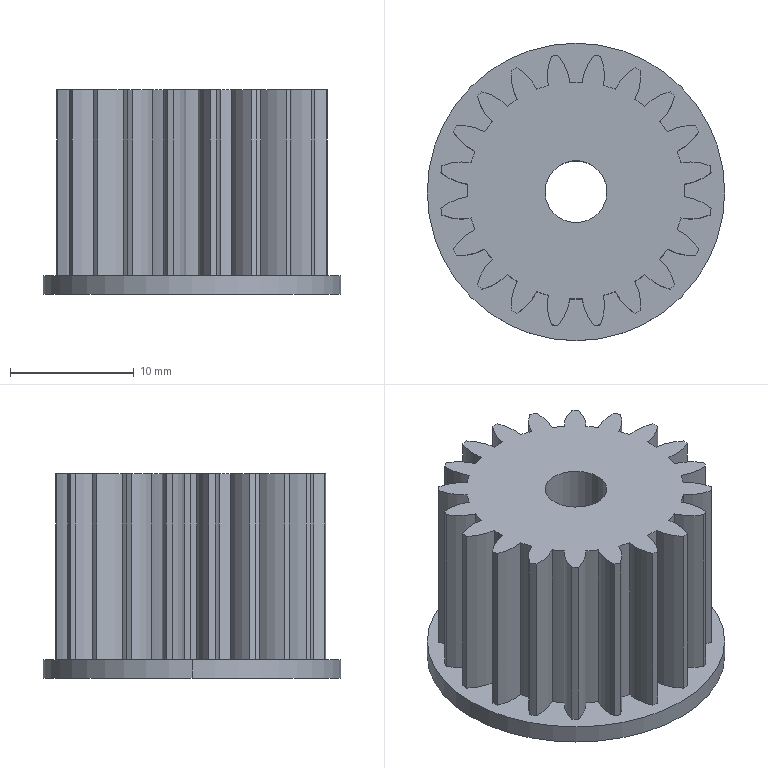Part | SolidWorks | features ICE 3, Extrusion 1 | 1 solid | 95 faces | box 24 x 24 x 16.5 mm | volume 4627 mm3 | cylinder 91 | plane 4 | commonest cylinder face diameters 8 x44 17.498 x21 22 x20 5 x2 14 x2 24 x2